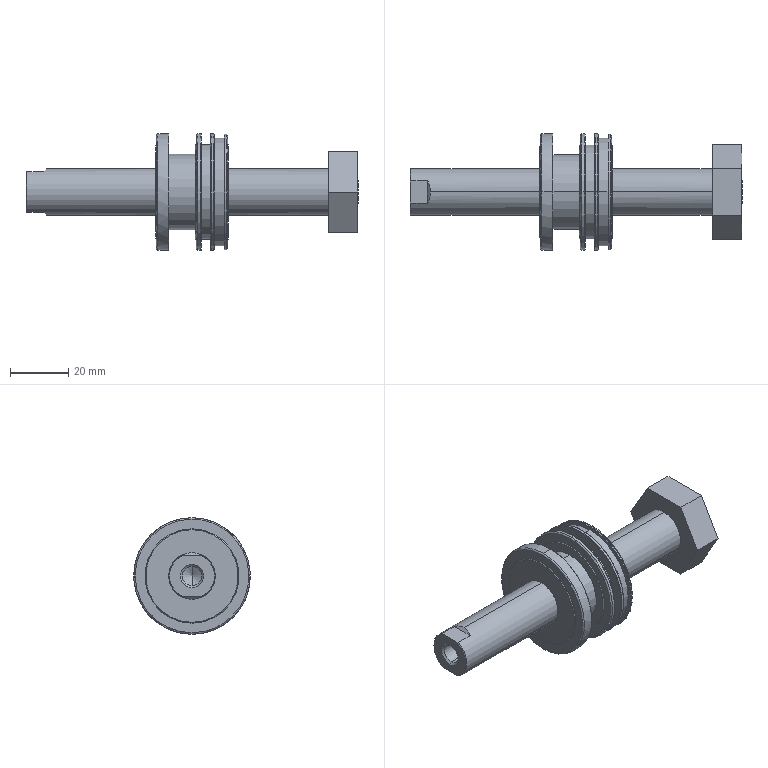Part | STEP file | ASND-0110-ACQDS-40x25-G-22aq | 2 solids | 87 faces | box 114 x 40 x 40 mm | volume 43729 mm3 | plane 29 | cylinder 24 | cone 20 | torus 14 | commonest cylinder face diameters 16 x6 40 x6 6.647 x4 25.8 x2 32.4 x2 37 x2